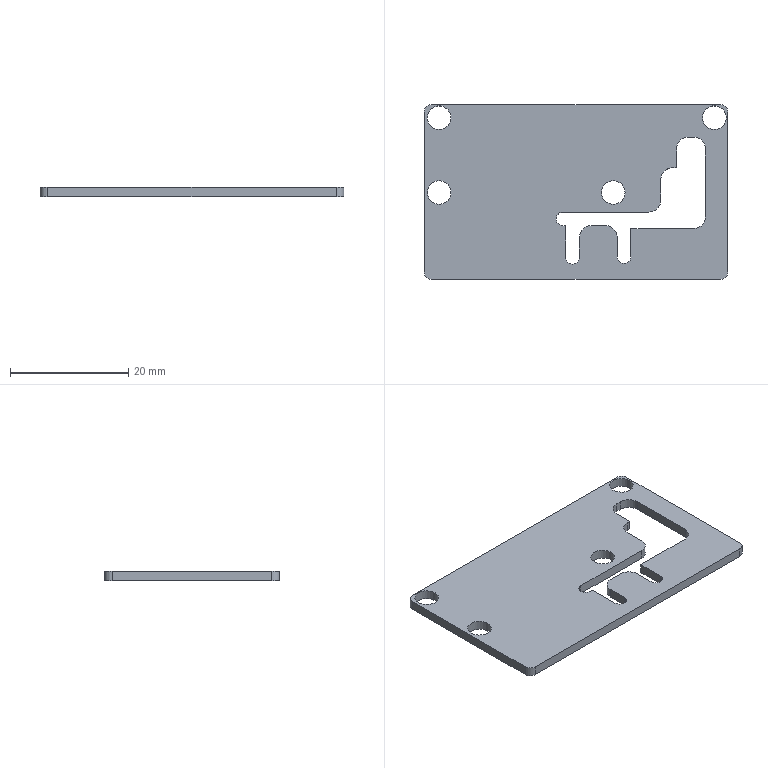Part | STEP file | Front stage control PCB | 1 solid | 70 faces | box 51.4 x 29.58 x 1.6 mm | volume 2071 mm3 | plane 55 | cylinder 15 | commonest cylinder face diameters 4 x11 2.54 x4